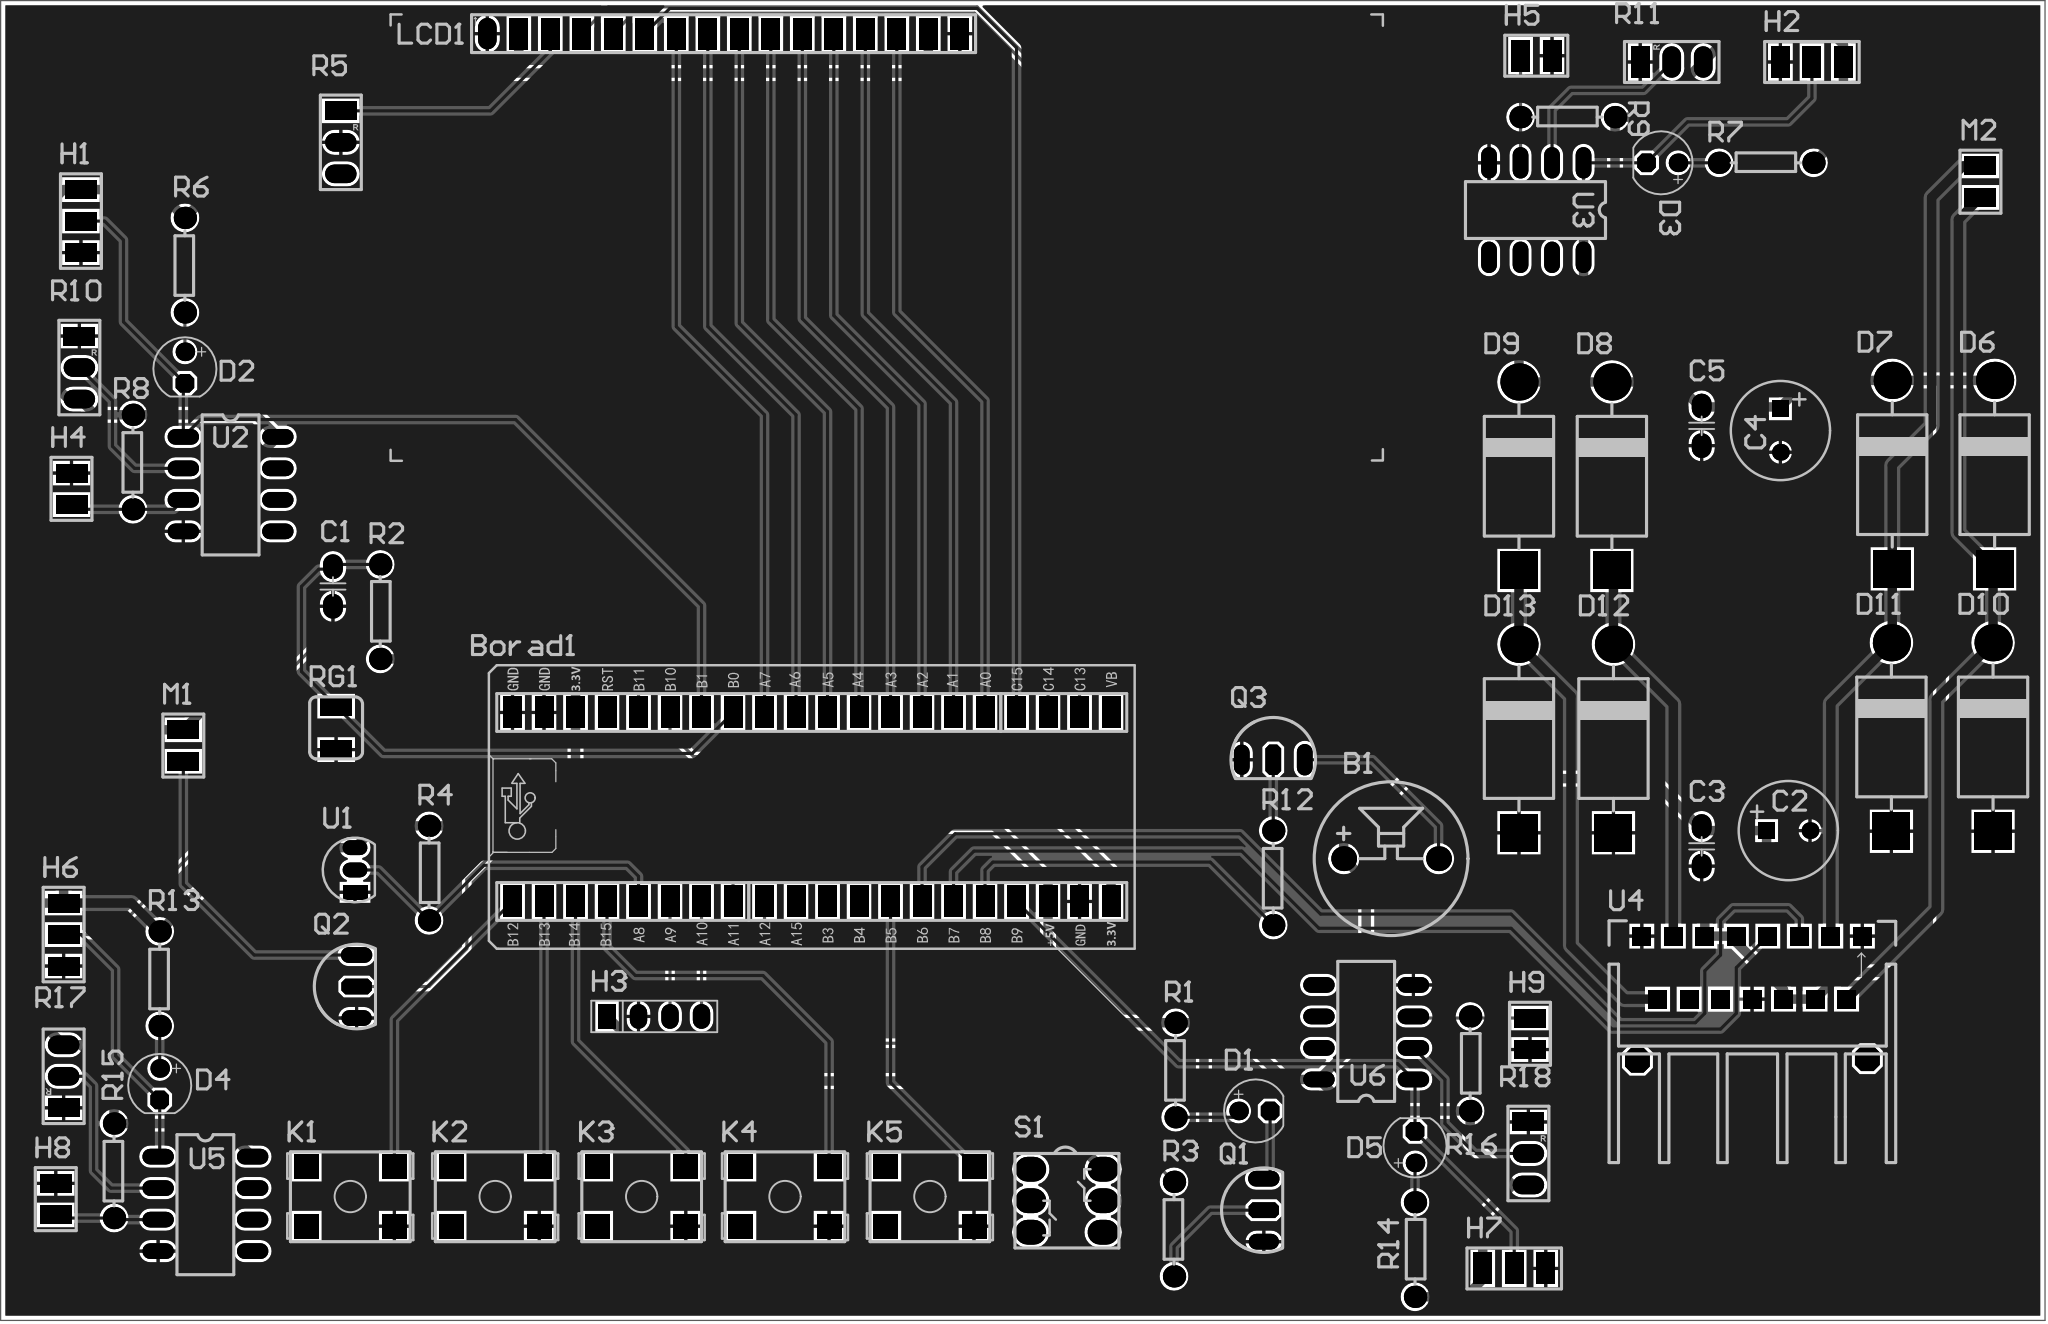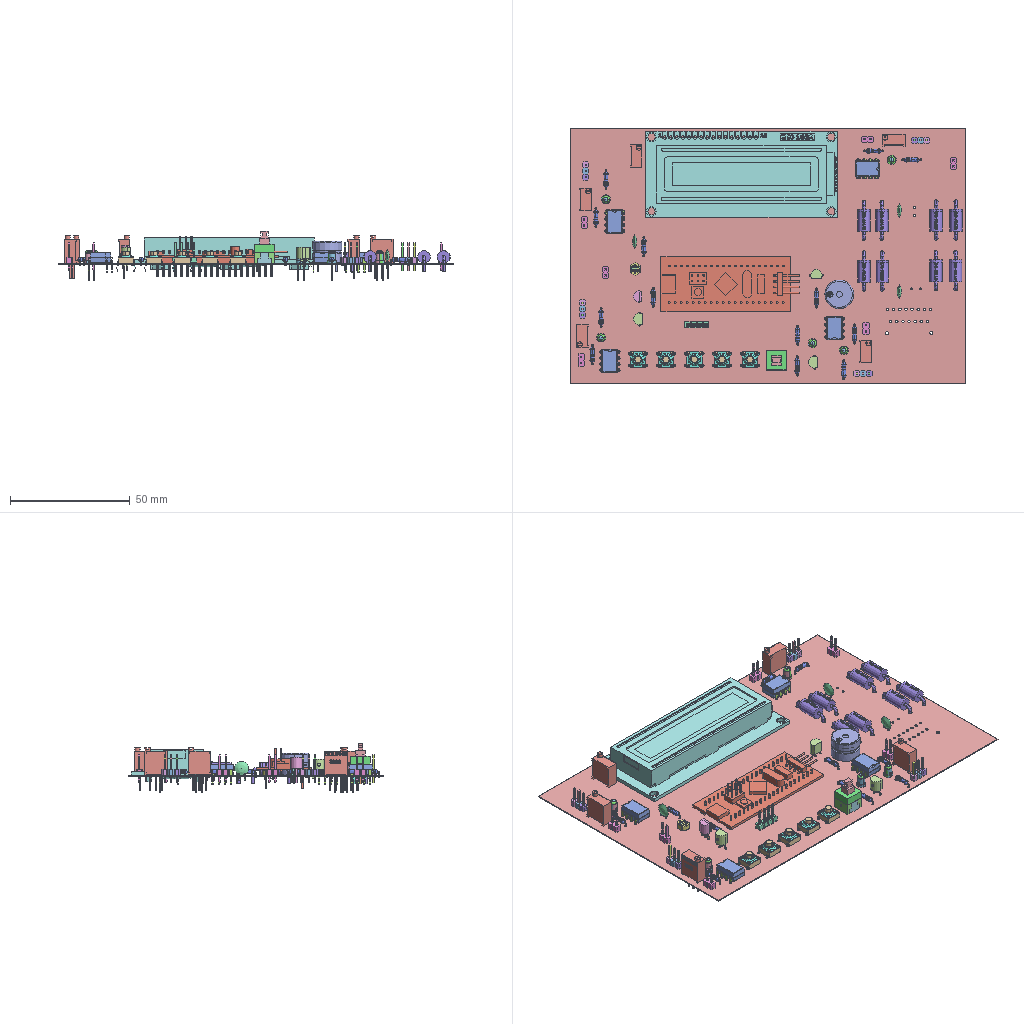Circuit board layout | Altium Designer | box 164.8 x 106.4 x 20.8 mm
Layer stack:
# Altium Designer layer stack of  (unit mm; dielectric type: 0 none, 1 core, 2 prepreg, 3 surface material)
index,name,kind,layer,copper_thickness_mm,dielectric_type,dielectric_thickness_mm,dielectric_material,dielectric_constant
0,Top Paste,other,,,,,,
1,Top Overlay,other,,,,,,
2,Top Solder,dielectric,,,3,0.0102,Solder Resist,3.5
3,Top Layer,copper,Top Layer,0.0356,,,,
4,Dielectric 1,dielectric,,,0,0.32,FR-4,4.8
5,Bottom Layer,copper,Bottom Layer,0.0356,,,,
6,Bottom Solder,dielectric,,,3,0.0102,Solder Resist,3.5
7,Bottom Overlay,other,,,,,,
8,Bottom Paste,other,,,,,,
# drill layer pairs: low layer,high layer
drill_pair,Top Layer,Bottom Layer
Part placement:
Designator,Comment,Layer,Footprint,Center-X(mm),Center-Y(mm),Rotation
U6,LM358,TopLayer,DIP8,135.509,43.815,180
U5,LM358,TopLayer,DIP8,41.91,29.972,0
U4,L298N-DIP,TopLayer,L298N,166.649,46.558,180
U3,LM358,TopLayer,DIP8,149.225,110.109,270
U2,LM358,TopLayer,DIP8,43.942,88.011,0
U1,DS18B20,TopLayer,DS18B20,53.975,56.896,90
S1,Latching switch,TopLayer,Switch,111.379,30.226,0
RG1,1M,TopLayer,RG,52.451,68.354,180
R18,10K,TopLayer,Res_Variable-DIP,148.59,34.036,360
R17,10K,TopLayer,Res_Variable-DIP,30.48,40.259,180
R16,1M,TopLayer,Resistor-7.62mm,143.891,41.275,270
R15,1M,TopLayer,Resistor-7.62mm,34.544,32.639,90
R14,300R,TopLayer,Resistor-7.62mm,139.446,26.289,270
R13,300R,TopLayer,Resistor-7.62mm,38.227,48.133,90
R12,1K,TopLayer,Resistor-7.62mm,128.016,56.261,90
R11,10K,TopLayer,Res_Variable-DIP,160.147,122.047,90
R10,10K,TopLayer,Res_Variable-DIP,31.75,97.409,360
R9,1M,TopLayer,Resistor-7.62mm,151.765,117.602,360
R8,1M,TopLayer,Resistor-7.62mm,36.068,89.789,90
R7,300R,TopLayer,Resistor-7.62mm,167.767,113.919,360
R6,300R,TopLayer,Resistor-7.62mm,40.259,105.664,90
R5,10K,TopLayer,Res_Variable-DIP,52.832,115.57,0
R4,10K,TopLayer,Resistor-7.62mm,59.944,56.642,270
R3,1K,TopLayer,Resistor-7.62mm,120.015,27.94,90
R2,10K,TopLayer,Resistor-7.62mm,56.007,77.724,270
R1,330R,TopLayer,Resistor-7.62mm,120.142,40.767,90
Q3,NPN,TopLayer,NPN_&_PNP,128.016,65.786,270
Q2,NPN,TopLayer,NPN_&_PNP,54.102,47.498,0
Q1,NPN,TopLayer,NPN_&_PNP,127.254,29.464,0
M2,MOTTOR,TopLayer,CON2,185.039,112.395,360
M1,FAN,TopLayer,CON2,40.132,66.929,0
LCD1,LCD1602,TopLayer,LCD1602,83.693,124.333,360
K5,Key,TopLayer,Buttom,100.33,30.594,180
K4,Key,TopLayer,Buttom,88.646,30.594,180
K3,Key,TopLayer,Buttom,77.089,30.594,180
K2,Key,TopLayer,Buttom,65.278,30.594,180
K1,Key,TopLayer,Buttom,53.594,30.594,180
H9,CON2,TopLayer,CON2,148.717,43.688,180
H8,CON2,TopLayer,CON2,29.845,30.353,0
H7,CON3,TopLayer,CON3,147.447,24.765,90
H6,CON3,TopLayer,CON3,30.48,51.689,0
H5,CON2,TopLayer,CON2,149.225,122.555,270
H4,CON2,TopLayer,CON2,31.115,87.63,0
H3,Program download interface,TopLayer,CON4,78.105,45.085,90
H2,CON3,TopLayer,CON3,171.45,122.047,270
H1,CON3,TopLayer,CON3,31.877,109.22,360
D13,1N4007,TopLayer,DIODE_-_15.24mm,147.828,67.495,270
D12,1N4007,TopLayer,DIODE_-_15.24mm,155.448,67.495,270
D11,1N4007,TopLayer,DIODE_-_15.24mm,177.86,67.622,270
D10,1N4007,TopLayer,DIODE_-_15.24mm,186.055,67.622,270
D9,1N4007,TopLayer,DIODE_-_15.24mm,147.828,88.646,270
D8,1N4007,TopLayer,DIODE_-_15.24mm,155.321,88.646,270
D7,1N4007,TopLayer,DIODE_-_15.24mm,177.927,88.773,270
D6,1N4007,TopLayer,DIODE_-_15.24mm,186.182,88.773,270
D5,LED,TopLayer,LED-3MM,139.446,34.544,270
D4,LED,TopLayer,LED-3MM,38.227,39.624,90
D3,LED,TopLayer,LED-3MM,159.385,113.919,360
D2,LED,TopLayer,LED-3MM,40.259,97.409,90
D1,LED,TopLayer,LED-3MM,126.492,37.465,180
C5,0.1uF,TopLayer,CAP_-_2.54mm,162.56,92.71,90
C4,220uF,TopLayer,CAPe_-_3.5MM,168.91,92.329,270
C3,0.1uF,TopLayer,CAP_-_2.54mm,162.56,58.801,90
C2,220uF,TopLayer,CAPe_-_3.5MM,169.545,60.071,0
C1,0.1uF,TopLayer,CAP_-_2.54mm,52.197,79.756,90
Borad1,STM32F103C6T6_Borad,TopLayer,STM32F103C8T6_买的,90.805,61.976,360
B1,Buzzer,TopLayer,BUZZER,137.518,57.808,0
Pad and via stacks:
# Altium Designer via and pad stacks of  (unit mm). Each distinct definition once, with the count of objects using it.
# via: kind,start_layer,end_layer,hole_mm,diameter_mm,mode(0 simple;1 top-mid-bottom;2 full stack),diameter_per_layer,count,example_net
# pad: kind,layer,hole_mm,hole_type(0 round;1 square;2 slot),plating,top_size,top_shape(1 round;2 rect;3 octagon;9 rounded rect),mid_size,bottom_size,mode,footprint,size_per_layer,count,example
pad,Multi-Layer,1,0,plated,2.54x1.5,2,2.54x1.5,2.54x1.5,0,LCD1602,,15,LCD1.14
pad,Multi-Layer,1,0,plated,2.54x1.5,1,2.54x1.5,2.54x1.5,0,LCD1602,,1,LCD1.1
pad,Multi-Layer,0.8,0,plated,1.8x1.8,1,1.8x1.8,1.8x1.8,0,Resistor-7.62mm,,26,R14.1
pad,Multi-Layer,0.8,0,plated,1.5x1.5,1,1.5x1.5,1.5x1.5,0,LED-3MM,,5,D5.2
pad,Multi-Layer,0.8,0,plated,1.5x1.5,3,1.5x1.5,1.5x1.5,0,LED-3MM,,5,D5.1
pad,Multi-Layer,0.8,0,plated,2.54x1.27,1,2.54x1.27,2.54x1.27,0,DIP8,,32,U6.1
pad,Multi-Layer,1,0,plated,2.54x1.5,2,2.54x1.5,2.54x1.5,0,CON2,,12,H9.2
pad,Multi-Layer,0.85,0,plated,1.35x1.35,2,1.35x1.35,1.35x1.35,0,CAPe - 3.5MM,,2,C4.1
pad,Multi-Layer,0.85,0,plated,1.35x1.35,1,1.35x1.35,1.35x1.35,0,CAPe - 3.5MM,,2,C4.2
pad,Multi-Layer,0.85,0,plated,2x2,1,2x2,2x2,0,BUZZER,,2,B1.2
pad,Multi-Layer,0.8,0,plated,1.27x2.54,1,1.27x2.54,1.27x2.54,0,NPN & PNP,,3,Q1.3
pad,Multi-Layer,0.8,0,plated,1.27x2.45,3,1.27x2.45,1.27x2.45,0,NPN & PNP,,3,Q1.1
pad,Multi-Layer,0.8,0,plated,1.27x2.45,1,1.27x2.45,1.27x2.45,0,NPN & PNP,,3,Q1.2
pad,Multi-Layer,0.7,0,plated,2x1.6,1,2x1.6,2x1.6,0,CAP - 2.54mm,,6,C5.1
pad,Multi-Layer,1,0,plated,2x2,2,2x2,2x2,0,Buttom,,20,K1.4
pad,Multi-Layer,0.8,0,plated,2x1.2,2,2x1.2,2x1.2,0,DS18B20,,1,U1.1
pad,Multi-Layer,0.8,0,plated,2x1.2,1,2x1.2,2x1.2,0,DS18B20,,2,U1.2
pad,Multi-Layer,0.8,0,plated,2.54x1.5,2,2.54x1.5,2.54x1.5,0,RG,,2,RG1.1
pad,Multi-Layer,1,0,plated,2.54x1.5,1,2.54x1.5,2.54x1.5,0,Res_Variable-DIP,,10,R5.3
pad,Multi-Layer,1,0,plated,2.54x1.5,2,2.54x1.5,2.54x1.5,0,Res_Variable-DIP,,5,R5.1
pad,Multi-Layer,1,0,plated,2.54x1.5,2,2.54x1.5,2.54x1.5,0,CON3,,12,H1.1
pad,Multi-Layer,1,0,plated,1.5x2.54,2,1.5x2.54,1.5x2.54,0,STM32F103C8T6_\u00C2\u00F2\u00B5\u00C4,,40,Borad1.25
pad,Multi-Layer,1,0,plated,1.4x2,2,1.4x2,1.4x2,0,CON4,,1,H3.1
pad,Multi-Layer,1,0,plated,1.4x2,1,1.4x2,1.4x2,0,CON4,,3,H3.2
pad,Multi-Layer,1,0,plated,2.5x2,1,2.5x2,2.5x2,0,Switch,,6,S1.6
pad,Multi-Layer,1.6,0,plated,3x3,2,3x3,3x3,0,DIODE - 15.24mm,,8,D9.1
pad,Multi-Layer,1.6,0,plated,3x3,1,3x3,3x3,0,DIODE - 15.24mm,,8,D9.2
pad,Multi-Layer,1.3,0,plated,2x2,3,2x2,2x2,0,L298N,,2,U4.0
pad,Multi-Layer,1,0,plated,1.524x1.524,2,1.524x1.524,1.524x1.524,0,L298N,,15,U4.1
Copper pours:
name,layer,net,type(0 solid;1 hatched;2 none)
G,Bottom Layer,GND,0
G,Top Layer,GND,0
Design rules, without the lines most boards share:
# Altium Designer design rules of  (exported by Altium Designer, unit mm)
# columns: name | kind | enabled | priority | scope1 | scope2 | descriptor | typed fields (field=value)
SilkToSilkClearance | 55 | enabled | 1 | All | All | Silk to Silk (Clearance=0mil) (All),(All) |
SilkToSolderMaskClearance | 54 | enabled | 1 | IsPad | All | Silk To Solder Mask (Clearance=0mil) (IsPad),(All) |
MinimumSolderMaskSliver | 53 | enabled | 1 | All | All | Minimum Solder Mask Sliver (Gap=0mil) (All),(All) |
HoleToHoleClearance | 52 | enabled | 1 | All | All | Hole To Hole Clearance (Gap=10mil) (All),(All) | gap=0.254
DiffPairsRouting | 51 | enabled | 1 | All | All | Differential Pairs Uncoupled Length using the Gap Constraints (Min=10mil) (Max=10mil) (Prefered=10mil)  and Width Constraints (Min=15mil) (Max=15mil) (Prefered=15mil) (All) |
SolderMaskExpansion | 13 | enabled | 1 | All | All | Solder Mask Expansion (Expansion =4mil) (All) | expansion=0.1016
PasteMaskExpansion | 14 | enabled | 1 | All | All | Paste Mask Expansion (Expansion =0mil) (All) | expansion=0
RoutingVias | 11 | enabled | 1 | All | All | Routing Via (MinHoleWidth=28mil) (MaxHoleWidth=28mil) (PreferredHoleWidth=28mil) (MinWidth=50mil) (MaxWidth=50mil) (PreferedWidth=50mil) (All) | via_min_hole=0.7112 via_max_hole=0.7112 via_preferred_diameter=1.27 via_preferred_hole=0.7112
Width | 2 | enabled | 1 | All | All | Width Constraint (Min=10mil) (Max=50mil) (Preferred=10mil) (All) |
PolygonConnect | 20 | enabled | 1 | All | All | Polygon Connect Rule(Relief Connect )(Conductor Width=10mil) (Relief Angle=90 Angle) (Entries=4) (Air Gap Width=10mil) (All),(All) | connect_style(0=relief,1=direct,2=none)=0 relief_conductor_width=0.254 relief_entries=4
PlaneConnect | 6 | enabled | 1 | All | All | Power Plane Connect Rule(Relief Connect )(Expansion=20mil) (Conductor Width=10mil) (Air Gap=10mil) (Entries=4) (All) | relief_conductor_width=0.254 relief_entries=4 relief_expansion=0.508
Clearance | 0 | enabled | 1 | All | All | Clearance Constraint (Gap=10mil) (All),(All) | gap=0.254